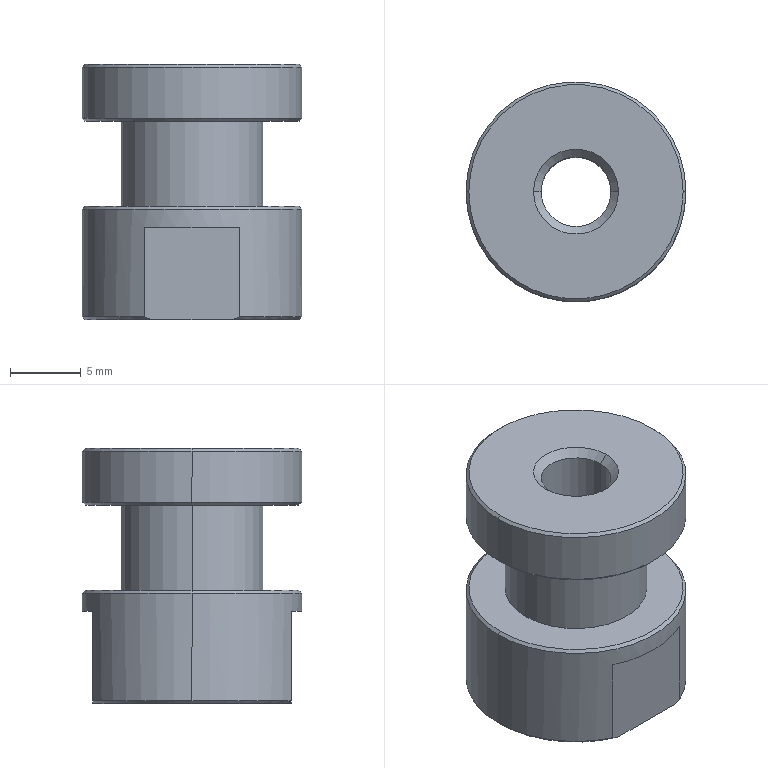Part | SolidWorks | features BaseBody 1 | 1 solid | 29 faces | box 15.5 x 15.5 x 18 mm | volume 2342 mm3 | cone 13 | cylinder 8 | plane 8 | commonest cylinder face diameters 15.5 x4 4.917 x2 10 x2
STEP:
#1=CARTESIAN_POINT('',(-2.458,0.,-17.459));
#2=VERTEX_POINT('',#1);
#3=CARTESIAN_POINT('',(2.458,0.,-17.459));
#4=VERTEX_POINT('',#3);
#5=CARTESIAN_POINT('',(0.,0.,-17.459));
#6=DIRECTION('',(0.,0.,1.));
#7=DIRECTION('',(1.,0.,0.));
#8=AXIS2_PLACEMENT_3D('',#5,#6,#7);
#9=CIRCLE('',#8,2.458);
#10=EDGE_CURVE('',#2,#4,#9,.T.);
#11=ORIENTED_EDGE('',*,*,#10,.T.);
#12=CARTESIAN_POINT('',(3.,0.,-18.));
#13=VERTEX_POINT('',#12);
#14=CARTESIAN_POINT('',(2.458,0.,-17.459));
#15=DIRECTION('',(0.7071,0.,-0.7071));
#16=VECTOR('',#15,1000.);
#17=LINE('',#14,#16);
#18=EDGE_CURVE('',#4,#13,#17,.T.);
#19=ORIENTED_EDGE('',*,*,#18,.T.);
#20=CARTESIAN_POINT('',(-3.,0.,-18.));
#21=VERTEX_POINT('',#20);
#22=CARTESIAN_POINT('',(0.,0.,-18.));
#23=DIRECTION('',(0.,0.,1.));
#24=DIRECTION('',(1.,0.,0.));
#25=AXIS2_PLACEMENT_3D('',#22,#23,#24);
#26=CIRCLE('',#25,3.);
#27=EDGE_CURVE('',#21,#13,#26,.T.);
#28=ORIENTED_EDGE('',*,*,#27,.F.);
#29=CARTESIAN_POINT('',(-2.458,0.,-17.459));
#30=DIRECTION('',(-0.7071,0.,-0.7071));
#31=VECTOR('',#30,1000.);
#32=LINE('',#29,#31);
#33=EDGE_CURVE('',#2,#21,#32,.T.);
#34=ORIENTED_EDGE('',*,*,#33,.F.);
#35=EDGE_LOOP('',(#11,#19,#28,#34));
#36=FACE_OUTER_BOUND('',#35,.T.);
#37=CARTESIAN_POINT('',(0.,0.,-17.459));
#38=DIRECTION('',(0.,0.,-1.));
#39=DIRECTION('',(-1.,0.,0.));
#40=AXIS2_PLACEMENT_3D('',#37,#38,#39);
#41=CONICAL_SURFACE('',#40,2.458,0.7854);
#42=ADVANCED_FACE('',(#36),#41,.F.);
#43=ORIENTED_EDGE('',*,*,#10,.F.);
#44=CARTESIAN_POINT('',(-2.458,0.,-0.5415));
#45=VERTEX_POINT('',#44);
#46=CARTESIAN_POINT('',(-2.458,0.,-50.));
#47=DIRECTION('',(0.,0.,1.));
#48=VECTOR('',#47,1000.);
#49=LINE('',#46,#48);
#50=EDGE_CURVE('',#2,#45,#49,.T.);
#51=ORIENTED_EDGE('',*,*,#50,.T.);
#52=CARTESIAN_POINT('',(2.458,0.,-0.5415));
#53=VERTEX_POINT('',#52);
#54=CARTESIAN_POINT('',(0.,0.,-0.5415));
#55=DIRECTION('',(0.,0.,1.));
#56=DIRECTION('',(1.,0.,0.));
#57=AXIS2_PLACEMENT_3D('',#54,#55,#56);
#58=CIRCLE('',#57,2.458);
#59=EDGE_CURVE('',#45,#53,#58,.T.);
#60=ORIENTED_EDGE('',*,*,#59,.T.);
#61=CARTESIAN_POINT('',(2.458,0.,-50.));
#62=DIRECTION('',(0.,0.,1.));
#63=VECTOR('',#62,1000.);
#64=LINE('',#61,#63);
#65=EDGE_CURVE('',#4,#53,#64,.T.);
#66=ORIENTED_EDGE('',*,*,#65,.F.);
#67=EDGE_LOOP('',(#43,#51,#60,#66));
#68=FACE_OUTER_BOUND('',#67,.T.);
#69=CARTESIAN_POINT('',(0.,0.,-50.));
#70=DIRECTION('',(0.,0.,1.));
#71=DIRECTION('',(1.,0.,0.));
#72=AXIS2_PLACEMENT_3D('',#69,#70,#71);
#73=CYLINDRICAL_SURFACE('',#72,2.458);
#74=ADVANCED_FACE('',(#68),#73,.F.);
#75=ORIENTED_EDGE('',*,*,#59,.F.);
#76=CARTESIAN_POINT('',(-3.,0.,0.));
#77=VERTEX_POINT('',#76);
#78=CARTESIAN_POINT('',(-3.,0.,0.));
#79=DIRECTION('',(-0.7071,0.,0.7071));
#80=VECTOR('',#79,1000.);
#81=LINE('',#78,#80);
#82=EDGE_CURVE('',#45,#77,#81,.T.);
#83=ORIENTED_EDGE('',*,*,#82,.T.);
#84=CARTESIAN_POINT('',(3.,0.,0.));
#85=VERTEX_POINT('',#84);
#86=CARTESIAN_POINT('',(0.,0.,0.));
#87=DIRECTION('',(0.,0.,1.));
#88=DIRECTION('',(1.,0.,0.));
#89=AXIS2_PLACEMENT_3D('',#86,#87,#88);
#90=CIRCLE('',#89,3.);
#91=EDGE_CURVE('',#77,#85,#90,.T.);
#92=ORIENTED_EDGE('',*,*,#91,.T.);
#93=CARTESIAN_POINT('',(3.,0.,0.));
#94=DIRECTION('',(0.7071,0.,0.7071));
#95=VECTOR('',#94,1000.);
#96=LINE('',#93,#95);
#97=EDGE_CURVE('',#53,#85,#96,.T.);
#98=ORIENTED_EDGE('',*,*,#97,.F.);
#99=EDGE_LOOP('',(#75,#83,#92,#98));
#100=FACE_OUTER_BOUND('',#99,.T.);
#101=CARTESIAN_POINT('',(0.,0.,0.));
#102=DIRECTION('',(0.,0.,1.));
#103=DIRECTION('',(1.,0.,0.));
#104=AXIS2_PLACEMENT_3D('',#101,#102,#103);
#105=CONICAL_SURFACE('',#104,3.,0.7854);
#106=ADVANCED_FACE('',(#100),#105,.F.);
#107=CARTESIAN_POINT('',(2.829,-7.,-18.));
#108=VERTEX_POINT('',#107);
#109=CARTESIAN_POINT('',(7.55,0.,-18.));
#110=VERTEX_POINT('',#109);
#111=CARTESIAN_POINT('',(0.,0.,-18.));
#112=DIRECTION('',(0.,0.,1.));
#113=DIRECTION('',(1.,0.,0.));
#114=AXIS2_PLACEMENT_3D('',#111,#112,#113);
#115=CIRCLE('',#114,7.55);
#116=EDGE_CURVE('',#108,#110,#115,.T.);
#117=ORIENTED_EDGE('',*,*,#116,.T.);
#118=CARTESIAN_POINT('',(7.75,0.,-17.8));
#119=VERTEX_POINT('',#118);
#120=CARTESIAN_POINT('',(7.75,0.,-17.8));
#121=DIRECTION('',(0.7071,0.,0.7071));
#122=VECTOR('',#121,1000.);
#123=LINE('',#120,#122);
#124=EDGE_CURVE('',#110,#119,#123,.T.);
#125=ORIENTED_EDGE('',*,*,#124,.T.);
#126=CARTESIAN_POINT('',(3.326,-7.,-17.8));
#127=VERTEX_POINT('',#126);
#128=CARTESIAN_POINT('',(0.,0.,-17.8));
#129=DIRECTION('',(0.,0.,1.));
#130=DIRECTION('',(1.,0.,0.));
#131=AXIS2_PLACEMENT_3D('',#128,#129,#130);
#132=CIRCLE('',#131,7.75);
#133=EDGE_CURVE('',#127,#119,#132,.T.);
#134=ORIENTED_EDGE('',*,*,#133,.F.);
#135=CARTESIAN_POINT('',(2.829,-7.,-18.));
#136=CARTESIAN_POINT('',(2.996,-7.,-17.937));
#137=CARTESIAN_POINT('',(3.161,-7.,-17.871));
#138=CARTESIAN_POINT('',(3.326,-7.,-17.8));
#139=B_SPLINE_CURVE_WITH_KNOTS('',3,(#135,#136,#137,#138),.UNSPECIFIED.,.F.,.F.,(4,4),(0.01089,0.01141),.UNSPECIFIED.);
#140=EDGE_CURVE('',#108,#127,#139,.T.);
#141=ORIENTED_EDGE('',*,*,#140,.F.);
#142=EDGE_LOOP('',(#117,#125,#134,#141));
#143=FACE_OUTER_BOUND('',#142,.T.);
#144=CARTESIAN_POINT('',(0.,0.,-17.8));
#145=DIRECTION('',(0.,0.,1.));
#146=DIRECTION('',(1.,0.,0.));
#147=AXIS2_PLACEMENT_3D('',#144,#145,#146);
#148=CONICAL_SURFACE('',#147,7.75,0.7854);
#149=ADVANCED_FACE('',(#143),#148,.T.);
#150=CARTESIAN_POINT('',(-3.326,7.,-17.8));
#151=VERTEX_POINT('',#150);
#152=CARTESIAN_POINT('',(-7.75,0.,-17.8));
#153=VERTEX_POINT('',#152);
#154=CARTESIAN_POINT('',(0.,0.,-17.8));
#155=DIRECTION('',(0.,0.,1.));
#156=DIRECTION('',(1.,0.,0.));
#157=AXIS2_PLACEMENT_3D('',#154,#155,#156);
#158=CIRCLE('',#157,7.75);
#159=EDGE_CURVE('',#151,#153,#158,.T.);
#160=ORIENTED_EDGE('',*,*,#159,.T.);
#161=CARTESIAN_POINT('',(-7.75,0.,-10.2));
#162=VERTEX_POINT('',#161);
#163=CARTESIAN_POINT('',(-7.75,0.,-50.));
#164=DIRECTION('',(0.,0.,1.));
#165=VECTOR('',#164,1000.);
#166=LINE('',#163,#165);
#167=EDGE_CURVE('',#153,#162,#166,.T.);
#168=ORIENTED_EDGE('',*,*,#167,.T.);
#169=CARTESIAN_POINT('',(7.75,0.,-10.2));
#170=VERTEX_POINT('',#169);
#171=CARTESIAN_POINT('',(0.,0.,-10.2));
#172=DIRECTION('',(0.,0.,1.));
#173=DIRECTION('',(1.,0.,0.));
#174=AXIS2_PLACEMENT_3D('',#171,#172,#173);
#175=CIRCLE('',#174,7.75);
#176=EDGE_CURVE('',#170,#162,#175,.T.);
#177=ORIENTED_EDGE('',*,*,#176,.F.);
#178=CARTESIAN_POINT('',(7.75,0.,-50.));
#179=DIRECTION('',(0.,0.,1.));
#180=VECTOR('',#179,1000.);
#181=LINE('',#178,#180);
#182=EDGE_CURVE('',#119,#170,#181,.T.);
#183=ORIENTED_EDGE('',*,*,#182,.F.);
#184=CARTESIAN_POINT('',(3.326,7.,-17.8));
#185=VERTEX_POINT('',#184);
#186=CARTESIAN_POINT('',(0.,0.,-17.8));
#187=DIRECTION('',(0.,0.,1.));
#188=DIRECTION('',(1.,0.,0.));
#189=AXIS2_PLACEMENT_3D('',#186,#187,#188);
#190=CIRCLE('',#189,7.75);
#191=EDGE_CURVE('',#119,#185,#190,.T.);
#192=ORIENTED_EDGE('',*,*,#191,.T.);
#193=CARTESIAN_POINT('',(3.326,7.,-11.5));
#194=VERTEX_POINT('',#193);
#195=CARTESIAN_POINT('',(3.326,7.,-11.5));
#196=DIRECTION('',(0.,0.,-1.));
#197=VECTOR('',#196,1000.);
#198=LINE('',#195,#197);
#199=EDGE_CURVE('',#194,#185,#198,.T.);
#200=ORIENTED_EDGE('',*,*,#199,.F.);
#201=CARTESIAN_POINT('',(-3.326,7.,-11.5));
#202=VERTEX_POINT('',#201);
#203=CARTESIAN_POINT('',(0.,0.,-11.5));
#204=DIRECTION('',(0.,0.,-1.));
#205=DIRECTION('',(1.,0.,0.));
#206=AXIS2_PLACEMENT_3D('',#203,#204,#205);
#207=CIRCLE('',#206,7.75);
#208=EDGE_CURVE('',#202,#194,#207,.T.);
#209=ORIENTED_EDGE('',*,*,#208,.F.);
#210=CARTESIAN_POINT('',(-3.326,7.,-11.5));
#211=DIRECTION('',(0.,0.,-1.));
#212=VECTOR('',#211,1000.);
#213=LINE('',#210,#212);
#214=EDGE_CURVE('',#202,#151,#213,.T.);
#215=ORIENTED_EDGE('',*,*,#214,.T.);
#216=EDGE_LOOP('',(#160,#168,#177,#183,#192,#200,#209,#215));
#217=FACE_OUTER_BOUND('',#216,.T.);
#218=CARTESIAN_POINT('',(0.,0.,-50.));
#219=DIRECTION('',(0.,0.,1.));
#220=DIRECTION('',(1.,0.,0.));
#221=AXIS2_PLACEMENT_3D('',#218,#219,#220);
#222=CYLINDRICAL_SURFACE('',#221,7.75);
#223=ADVANCED_FACE('',(#217),#222,.T.);
#224=CARTESIAN_POINT('',(7.55,0.,-10.));
#225=VERTEX_POINT('',#224);
#226=CARTESIAN_POINT('',(-7.55,0.,-10.));
#227=VERTEX_POINT('',#226);
#228=CARTESIAN_POINT('',(0.,0.,-10.));
#229=DIRECTION('',(0.,0.,1.));
#230=DIRECTION('',(1.,0.,0.));
#231=AXIS2_PLACEMENT_3D('',#228,#229,#230);
#232=CIRCLE('',#231,7.55);
#233=EDGE_CURVE('',#225,#227,#232,.T.);
#234=ORIENTED_EDGE('',*,*,#233,.F.);
#235=CARTESIAN_POINT('',(7.55,0.,-10.));
#236=DIRECTION('',(0.7071,0.,-0.7071));
#237=VECTOR('',#236,1000.);
#238=LINE('',#235,#237);
#239=EDGE_CURVE('',#225,#170,#238,.T.);
#240=ORIENTED_EDGE('',*,*,#239,.T.);
#241=ORIENTED_EDGE('',*,*,#176,.T.);
#242=CARTESIAN_POINT('',(-7.55,0.,-10.));
#243=DIRECTION('',(-0.7071,0.,-0.7071));
#244=VECTOR('',#243,1000.);
#245=LINE('',#242,#244);
#246=EDGE_CURVE('',#227,#162,#245,.T.);
#247=ORIENTED_EDGE('',*,*,#246,.F.);
#248=EDGE_LOOP('',(#234,#240,#241,#247));
#249=FACE_OUTER_BOUND('',#248,.T.);
#250=CARTESIAN_POINT('',(0.,0.,-10.));
#251=DIRECTION('',(0.,0.,-1.));
#252=DIRECTION('',(-1.,0.,0.));
#253=AXIS2_PLACEMENT_3D('',#250,#251,#252);
#254=CONICAL_SURFACE('',#253,7.55,0.7854);
#255=ADVANCED_FACE('',(#249),#254,.T.);
#256=CARTESIAN_POINT('',(5.,0.,-10.));
#257=VERTEX_POINT('',#256);
#258=CARTESIAN_POINT('',(-5.,0.,-10.));
#259=VERTEX_POINT('',#258);
#260=CARTESIAN_POINT('',(0.,0.,-10.));
#261=DIRECTION('',(0.,0.,1.));
#262=DIRECTION('',(1.,0.,0.));
#263=AXIS2_PLACEMENT_3D('',#260,#261,#262);
#264=CIRCLE('',#263,5.);
#265=EDGE_CURVE('',#257,#259,#264,.T.);
#266=ORIENTED_EDGE('',*,*,#265,.T.);
#267=CARTESIAN_POINT('',(-5.,0.,-4.));
#268=VERTEX_POINT('',#267);
#269=CARTESIAN_POINT('',(-5.,0.,-50.));
#270=DIRECTION('',(0.,0.,1.));
#271=VECTOR('',#270,1000.);
#272=LINE('',#269,#271);
#273=EDGE_CURVE('',#259,#268,#272,.T.);
#274=ORIENTED_EDGE('',*,*,#273,.T.);
#275=CARTESIAN_POINT('',(5.,0.,-4.));
#276=VERTEX_POINT('',#275);
#277=CARTESIAN_POINT('',(0.,0.,-4.));
#278=DIRECTION('',(0.,0.,1.));
#279=DIRECTION('',(1.,0.,0.));
#280=AXIS2_PLACEMENT_3D('',#277,#278,#279);
#281=CIRCLE('',#280,5.);
#282=EDGE_CURVE('',#276,#268,#281,.T.);
#283=ORIENTED_EDGE('',*,*,#282,.F.);
#284=CARTESIAN_POINT('',(5.,0.,-50.));
#285=DIRECTION('',(0.,0.,1.));
#286=VECTOR('',#285,1000.);
#287=LINE('',#284,#286);
#288=EDGE_CURVE('',#257,#276,#287,.T.);
#289=ORIENTED_EDGE('',*,*,#288,.F.);
#290=EDGE_LOOP('',(#266,#274,#283,#289));
#291=FACE_OUTER_BOUND('',#290,.T.);
#292=CARTESIAN_POINT('',(0.,0.,-50.));
#293=DIRECTION('',(0.,0.,1.));
#294=DIRECTION('',(1.,0.,0.));
#295=AXIS2_PLACEMENT_3D('',#292,#293,#294);
#296=CYLINDRICAL_SURFACE('',#295,5.);
#297=ADVANCED_FACE('',(#291),#296,.T.);
#298=CARTESIAN_POINT('',(7.55,0.,-4.));
#299=VERTEX_POINT('',#298);
#300=CARTESIAN_POINT('',(-7.55,0.,-4.));
#301=VERTEX_POINT('',#300);
#302=CARTESIAN_POINT('',(0.,0.,-4.));
#303=DIRECTION('',(0.,0.,1.));
#304=DIRECTION('',(1.,0.,0.));
#305=AXIS2_PLACEMENT_3D('',#302,#303,#304);
#306=CIRCLE('',#305,7.55);
#307=EDGE_CURVE('',#299,#301,#306,.T.);
#308=ORIENTED_EDGE('',*,*,#307,.T.);
#309=CARTESIAN_POINT('',(-7.75,0.,-3.8));
#310=VERTEX_POINT('',#309);
#311=CARTESIAN_POINT('',(-7.75,0.,-3.8));
#312=DIRECTION('',(-0.7071,0.,0.7071));
#313=VECTOR('',#312,1000.);
#314=LINE('',#311,#313);
#315=EDGE_CURVE('',#301,#310,#314,.T.);
#316=ORIENTED_EDGE('',*,*,#315,.T.);
#317=CARTESIAN_POINT('',(7.75,0.,-3.8));
#318=VERTEX_POINT('',#317);
#319=CARTESIAN_POINT('',(0.,0.,-3.8));
#320=DIRECTION('',(0.,0.,1.));
#321=DIRECTION('',(1.,0.,0.));
#322=AXIS2_PLACEMENT_3D('',#319,#320,#321);
#323=CIRCLE('',#322,7.75);
#324=EDGE_CURVE('',#318,#310,#323,.T.);
#325=ORIENTED_EDGE('',*,*,#324,.F.);
#326=CARTESIAN_POINT('',(7.75,0.,-3.8));
#327=DIRECTION('',(0.7071,0.,0.7071));
#328=VECTOR('',#327,1000.);
#329=LINE('',#326,#328);
#330=EDGE_CURVE('',#299,#318,#329,.T.);
#331=ORIENTED_EDGE('',*,*,#330,.F.);
#332=EDGE_LOOP('',(#308,#316,#325,#331));
#333=FACE_OUTER_BOUND('',#332,.T.);
#334=CARTESIAN_POINT('',(0.,0.,-3.8));
#335=DIRECTION('',(0.,0.,1.));
#336=DIRECTION('',(1.,0.,0.));
#337=AXIS2_PLACEMENT_3D('',#334,#335,#336);
#338=CONICAL_SURFACE('',#337,7.75,0.7854);
#339=ADVANCED_FACE('',(#333),#338,.T.);
#340=ORIENTED_EDGE('',*,*,#324,.T.);
#341=CARTESIAN_POINT('',(-7.75,0.,-0.2));
#342=VERTEX_POINT('',#341);
#343=CARTESIAN_POINT('',(-7.75,0.,-50.));
#344=DIRECTION('',(0.,0.,1.));
#345=VECTOR('',#344,1000.);
#346=LINE('',#343,#345);
#347=EDGE_CURVE('',#310,#342,#346,.T.);
#348=ORIENTED_EDGE('',*,*,#347,.T.);
#349=CARTESIAN_POINT('',(7.75,0.,-0.2));
#350=VERTEX_POINT('',#349);
#351=CARTESIAN_POINT('',(0.,0.,-0.2));
#352=DIRECTION('',(0.,0.,1.));
#353=DIRECTION('',(1.,0.,0.));
#354=AXIS2_PLACEMENT_3D('',#351,#352,#353);
#355=CIRCLE('',#354,7.75);
#356=EDGE_CURVE('',#350,#342,#355,.T.);
#357=ORIENTED_EDGE('',*,*,#356,.F.);
#358=CARTESIAN_POINT('',(7.75,0.,-50.));
#359=DIRECTION('',(0.,0.,1.));
#360=VECTOR('',#359,1000.);
#361=LINE('',#358,#360);
#362=EDGE_CURVE('',#318,#350,#361,.T.);
#363=ORIENTED_EDGE('',*,*,#362,.F.);
#364=EDGE_LOOP('',(#340,#348,#357,#363));
#365=FACE_OUTER_BOUND('',#364,.T.);
#366=CARTESIAN_POINT('',(0.,0.,-50.));
#367=DIRECTION('',(0.,0.,1.));
#368=DIRECTION('',(1.,0.,0.));
#369=AXIS2_PLACEMENT_3D('',#366,#367,#368);
#370=CYLINDRICAL_SURFACE('',#369,7.75);
#371=ADVANCED_FACE('',(#365),#370,.T.);
#372=CARTESIAN_POINT('',(7.55,0.,0.));
#373=VERTEX_POINT('',#372);
#374=CARTESIAN_POINT('',(-7.55,0.,0.));
#375=VERTEX_POINT('',#374);
#376=CARTESIAN_POINT('',(0.,0.,0.));
#377=DIRECTION('',(0.,0.,1.));
#378=DIRECTION('',(1.,0.,0.));
#379=AXIS2_PLACEMENT_3D('',#376,#377,#378);
#380=CIRCLE('',#379,7.55);
#381=EDGE_CURVE('',#373,#375,#380,.T.);
#382=ORIENTED_EDGE('',*,*,#381,.F.);
#383=CARTESIAN_POINT('',(7.55,0.,0.));
#384=DIRECTION('',(0.7071,0.,-0.7071));
#385=VECTOR('',#384,1000.);
#386=LINE('',#383,#385);
#387=EDGE_CURVE('',#373,#350,#386,.T.);
#388=ORIENTED_EDGE('',*,*,#387,.T.);
#389=ORIENTED_EDGE('',*,*,#356,.T.);
#390=CARTESIAN_POINT('',(-7.55,0.,0.));
#391=DIRECTION('',(-0.7071,0.,-0.7071));
#392=VECTOR('',#391,1000.);
#393=LINE('',#390,#392);
#394=EDGE_CURVE('',#375,#342,#393,.T.);
#395=ORIENTED_EDGE('',*,*,#394,.F.);
#396=EDGE_LOOP('',(#382,#388,#389,#395));
#397=FACE_OUTER_BOUND('',#396,.T.);
#398=CARTESIAN_POINT('',(0.,0.,0.));
#399=DIRECTION('',(0.,0.,-1.));
#400=DIRECTION('',(-1.,0.,0.));
#401=AXIS2_PLACEMENT_3D('',#398,#399,#400);
#402=CONICAL_SURFACE('',#401,7.55,0.7854);
#403=ADVANCED_FACE('',(#397),#402,.T.);
#404=CARTESIAN_POINT('',(-3.326,-7.,-17.8));
#405=VERTEX_POINT('',#404);
#406=CARTESIAN_POINT('',(-2.829,-7.,-18.));
#407=VERTEX_POINT('',#406);
#408=CARTESIAN_POINT('',(-3.326,-7.,-17.8));
#409=CARTESIAN_POINT('',(-3.162,-7.,-17.87));
#410=CARTESIAN_POINT('',(-2.997,-7.,-17.937));
#411=CARTESIAN_POINT('',(-2.829,-7.,-18.));
#412=B_SPLINE_CURVE_WITH_KNOTS('',3,(#408,#409,#410,#411),.UNSPECIFIED.,.F.,.F.,(4,4),(0.004643,0.005176),.UNSPECIFIED.);
#413=EDGE_CURVE('',#405,#407,#412,.T.);
#414=ORIENTED_EDGE('',*,*,#413,.F.);
#415=CARTESIAN_POINT('',(0.,0.,-17.8));
#416=DIRECTION('',(0.,0.,1.));
#417=DIRECTION('',(1.,0.,0.));
#418=AXIS2_PLACEMENT_3D('',#415,#416,#417);
#419=CIRCLE('',#418,7.75);
#420=EDGE_CURVE('',#153,#405,#419,.T.);
#421=ORIENTED_EDGE('',*,*,#420,.F.);
#422=ORIENTED_EDGE('',*,*,#159,.F.);
#423=CARTESIAN_POINT('',(-2.829,7.,-18.));
#424=VERTEX_POINT('',#423);
#425=CARTESIAN_POINT('',(-2.829,7.,-18.));
#426=CARTESIAN_POINT('',(-2.996,7.,-17.937));
#427=CARTESIAN_POINT('',(-3.161,7.,-17.871));
#428=CARTESIAN_POINT('',(-3.326,7.,-17.8));
#429=B_SPLINE_CURVE_WITH_KNOTS('',3,(#425,#426,#427,#428),.UNSPECIFIED.,.F.,.F.,(4,4),(0.01089,0.01141),.UNSPECIFIED.);
#430=EDGE_CURVE('',#424,#151,#429,.T.);
#431=ORIENTED_EDGE('',*,*,#430,.F.);
#432=CARTESIAN_POINT('',(0.,0.,-18.));
#433=DIRECTION('',(0.,0.,1.));
#434=DIRECTION('',(1.,0.,0.));
#435=AXIS2_PLACEMENT_3D('',#432,#433,#434);
#436=CIRCLE('',#435,7.55);
#437=EDGE_CURVE('',#424,#407,#436,.T.);
#438=ORIENTED_EDGE('',*,*,#437,.T.);
#439=EDGE_LOOP('',(#414,#421,#422,#431,#438));
#440=FACE_OUTER_BOUND('',#439,.T.);
#441=CARTESIAN_POINT('',(0.,0.,-17.8));
#442=DIRECTION('',(0.,0.,1.));
#443=DIRECTION('',(1.,0.,0.));
#444=AXIS2_PLACEMENT_3D('',#441,#442,#443);
#445=CONICAL_SURFACE('',#444,7.75,0.7854);
#446=ADVANCED_FACE('',(#440),#445,.T.);
#447=CARTESIAN_POINT('',(0.,0.,0.));
#448=DIRECTION('',(0.,0.,1.));
#449=DIRECTION('',(1.,0.,0.));
#450=AXIS2_PLACEMENT_3D('',#447,#448,#449);
#451=CIRCLE('',#450,3.);
#452=EDGE_CURVE('',#85,#77,#451,.T.);
#453=ORIENTED_EDGE('',*,*,#452,.F.);
#454=ORIENTED_EDGE('',*,*,#91,.F.);
#455=EDGE_LOOP('',(#453,#454));
#456=FACE_BOUND('',#455,.T.);
#457=CARTESIAN_POINT('',(0.,0.,0.));
#458=DIRECTION('',(0.,0.,1.));
#459=DIRECTION('',(1.,0.,0.));
#460=AXIS2_PLACEMENT_3D('',#457,#458,#459);
#461=CIRCLE('',#460,7.55);
#462=EDGE_CURVE('',#375,#373,#461,.T.);
#463=ORIENTED_EDGE('',*,*,#462,.T.);
#464=ORIENTED_EDGE('',*,*,#381,.T.);
#465=EDGE_LOOP('',(#463,#464));
#466=FACE_OUTER_BOUND('',#465,.T.);
#467=CARTESIAN_POINT('',(0.,0.,0.));
#468=DIRECTION('',(0.,0.,1.));
#469=DIRECTION('',(1.,0.,0.));
#470=AXIS2_PLACEMENT_3D('',#467,#468,#469);
#471=PLANE('',#470);
#472=ADVANCED_FACE('',(#456,#466),#471,.T.);
#473=ORIENTED_EDGE('',*,*,#387,.F.);
#474=ORIENTED_EDGE('',*,*,#462,.F.);
#475=ORIENTED_EDGE('',*,*,#394,.T.);
#476=CARTESIAN_POINT('',(0.,0.,-0.2));
#477=DIRECTION('',(0.,0.,1.));
#478=DIRECTION('',(1.,0.,0.));
#479=AXIS2_PLACEMENT_3D('',#476,#477,#478);
#480=CIRCLE('',#479,7.75);
#481=EDGE_CURVE('',#342,#350,#480,.T.);
#482=ORIENTED_EDGE('',*,*,#481,.T.);
#483=EDGE_LOOP('',(#473,#474,#475,#482));
#484=FACE_OUTER_BOUND('',#483,.T.);
#485=CARTESIAN_POINT('',(0.,0.,0.));
#486=DIRECTION('',(0.,0.,-1.));
#487=DIRECTION('',(-1.,0.,0.));
#488=AXIS2_PLACEMENT_3D('',#485,#486,#487);
#489=CONICAL_SURFACE('',#488,7.55,0.7854);
#490=ADVANCED_FACE('',(#484),#489,.T.);
#491=ORIENTED_EDGE('',*,*,#347,.F.);
#492=CARTESIAN_POINT('',(0.,0.,-3.8));
#493=DIRECTION('',(0.,0.,1.));
#494=DIRECTION('',(1.,0.,0.));
#495=AXIS2_PLACEMENT_3D('',#492,#493,#494);
#496=CIRCLE('',#495,7.75);
#497=EDGE_CURVE('',#310,#318,#496,.T.);
#498=ORIENTED_EDGE('',*,*,#497,.T.);
#499=ORIENTED_EDGE('',*,*,#362,.T.);
#500=ORIENTED_EDGE('',*,*,#481,.F.);
#501=EDGE_LOOP('',(#491,#498,#499,#500));
#502=FACE_OUTER_BOUND('',#501,.T.);
#503=CARTESIAN_POINT('',(0.,0.,-50.));
#504=DIRECTION('',(0.,0.,1.));
#505=DIRECTION('',(1.,0.,0.));
#506=AXIS2_PLACEMENT_3D('',#503,#504,#505);
#507=CYLINDRICAL_SURFACE('',#506,7.75);
#508=ADVANCED_FACE('',(#502),#507,.T.);
#509=ORIENTED_EDGE('',*,*,#315,.F.);
#510=CARTESIAN_POINT('',(0.,0.,-4.));
#511=DIRECTION('',(0.,0.,1.));
#512=DIRECTION('',(1.,0.,0.));
#513=AXIS2_PLACEMENT_3D('',#510,#511,#512);
#514=CIRCLE('',#513,7.55);
#515=EDGE_CURVE('',#301,#299,#514,.T.);
#516=ORIENTED_EDGE('',*,*,#515,.T.);
#517=ORIENTED_EDGE('',*,*,#330,.T.);
#518=ORIENTED_EDGE('',*,*,#497,.F.);
#519=EDGE_LOOP('',(#509,#516,#517,#518));
#520=FACE_OUTER_BOUND('',#519,.T.);
#521=CARTESIAN_POINT('',(0.,0.,-3.8));
#522=DIRECTION('',(0.,0.,1.));
#523=DIRECTION('',(1.,0.,0.));
#524=AXIS2_PLACEMENT_3D('',#521,#522,#523);
#525=CONICAL_SURFACE('',#524,7.75,0.7854);
#526=ADVANCED_FACE('',(#520),#525,.T.);
#527=ORIENTED_EDGE('',*,*,#282,.T.);
#528=CARTESIAN_POINT('',(0.,0.,-4.));
#529=DIRECTION('',(0.,0.,1.));
#530=DIRECTION('',(1.,0.,0.));
#531=AXIS2_PLACEMENT_3D('',#528,#529,#530);
#532=CIRCLE('',#531,5.);
#533=EDGE_CURVE('',#268,#276,#532,.T.);
#534=ORIENTED_EDGE('',*,*,#533,.T.);
#535=EDGE_LOOP('',(#527,#534));
#536=FACE_BOUND('',#535,.T.);
#537=ORIENTED_EDGE('',*,*,#307,.F.);
#538=ORIENTED_EDGE('',*,*,#515,.F.);
#539=EDGE_LOOP('',(#537,#538));
#540=FACE_OUTER_BOUND('',#539,.T.);
#541=CARTESIAN_POINT('',(0.,7.55,-4.));
#542=DIRECTION('',(0.,0.,-1.));
#543=DIRECTION('',(-1.,0.,0.));
#544=AXIS2_PLACEMENT_3D('',#541,#542,#543);
#545=PLANE('',#544);
#546=ADVANCED_FACE('',(#536,#540),#545,.T.);
#547=ORIENTED_EDGE('',*,*,#273,.F.);
#548=CARTESIAN_POINT('',(0.,0.,-10.));
#549=DIRECTION('',(0.,0.,1.));
#550=DIRECTION('',(1.,0.,0.));
#551=AXIS2_PLACEMENT_3D('',#548,#549,#550);
#552=CIRCLE('',#551,5.);
#553=EDGE_CURVE('',#259,#257,#552,.T.);
#554=ORIENTED_EDGE('',*,*,#553,.T.);
#555=ORIENTED_EDGE('',*,*,#288,.T.);
#556=ORIENTED_EDGE('',*,*,#533,.F.);
#557=EDGE_LOOP('',(#547,#554,#555,#556));
#558=FACE_OUTER_BOUND('',#557,.T.);
#559=CARTESIAN_POINT('',(0.,0.,-50.));
#560=DIRECTION('',(0.,0.,1.));
#561=DIRECTION('',(1.,0.,0.));
#562=AXIS2_PLACEMENT_3D('',#559,#560,#561);
#563=CYLINDRICAL_SURFACE('',#562,5.);
#564=ADVANCED_FACE('',(#558),#563,.T.);
#565=CARTESIAN_POINT('',(0.,0.,-10.));
#566=DIRECTION('',(0.,0.,1.));
#567=DIRECTION('',(1.,0.,0.));
#568=AXIS2_PLACEMENT_3D('',#565,#566,#567);
#569=CIRCLE('',#568,7.55);
#570=EDGE_CURVE('',#227,#225,#569,.T.);
#571=ORIENTED_EDGE('',*,*,#570,.T.);
#572=ORIENTED_EDGE('',*,*,#233,.T.);
#573=EDGE_LOOP('',(#571,#572));
#574=FACE_OUTER_BOUND('',#573,.T.);
#575=ORIENTED_EDGE('',*,*,#265,.F.);
#576=ORIENTED_EDGE('',*,*,#553,.F.);
#577=EDGE_LOOP('',(#575,#576));
#578=FACE_BOUND('',#577,.T.);
#579=CARTESIAN_POINT('',(0.,5.,-10.));
#580=DIRECTION('',(0.,0.,1.));
#581=DIRECTION('',(1.,0.,0.));
#582=AXIS2_PLACEMENT_3D('',#579,#580,#581);
#583=PLANE('',#582);
#584=ADVANCED_FACE('',(#574,#578),#583,.T.);
#585=ORIENTED_EDGE('',*,*,#239,.F.);
#586=ORIENTED_EDGE('',*,*,#570,.F.);
#587=ORIENTED_EDGE('',*,*,#246,.T.);
#588=CARTESIAN_POINT('',(0.,0.,-10.2));
#589=DIRECTION('',(0.,0.,1.));
#590=DIRECTION('',(1.,0.,0.));
#591=AXIS2_PLACEMENT_3D('',#588,#589,#590);
#592=CIRCLE('',#591,7.75);
#593=EDGE_CURVE('',#162,#170,#592,.T.);
#594=ORIENTED_EDGE('',*,*,#593,.T.);
#595=EDGE_LOOP('',(#585,#586,#587,#594));
#596=FACE_OUTER_BOUND('',#595,.T.);
#597=CARTESIAN_POINT('',(0.,0.,-10.));
#598=DIRECTION('',(0.,0.,-1.));
#599=DIRECTION('',(-1.,0.,0.));
#600=AXIS2_PLACEMENT_3D('',#597,#598,#599);
#601=CONICAL_SURFACE('',#600,7.55,0.7854);
#602=ADVANCED_FACE('',(#596),#601,.T.);
#603=ORIENTED_EDGE('',*,*,#167,.F.);
#604=ORIENTED_EDGE('',*,*,#420,.T.);
#605=CARTESIAN_POINT('',(-3.326,-7.,-11.5));
#606=VERTEX_POINT('',#605);
#607=CARTESIAN_POINT('',(-3.326,-7.,-11.5));
#608=DIRECTION('',(0.,0.,-1.));
#609=VECTOR('',#608,1000.);
#610=LINE('',#607,#609);
#611=EDGE_CURVE('',#606,#405,#610,.T.);
#612=ORIENTED_EDGE('',*,*,#611,.F.);
#613=CARTESIAN_POINT('',(3.326,-7.,-11.5));
#614=VERTEX_POINT('',#613);
#615=CARTESIAN_POINT('',(0.,0.,-11.5));
#616=DIRECTION('',(0.,0.,-1.));
#617=DIRECTION('',(1.,0.,0.));
#618=AXIS2_PLACEMENT_3D('',#615,#616,#617);
#619=CIRCLE('',#618,7.75);
#620=EDGE_CURVE('',#614,#606,#619,.T.);
#621=ORIENTED_EDGE('',*,*,#620,.F.);
#622=CARTESIAN_POINT('',(3.326,-7.,-11.5));
#623=DIRECTION('',(0.,0.,-1.));
#624=VECTOR('',#623,1000.);
#625=LINE('',#622,#624);
#626=EDGE_CURVE('',#614,#127,#625,.T.);
#627=ORIENTED_EDGE('',*,*,#626,.T.);
#628=ORIENTED_EDGE('',*,*,#133,.T.);
#629=ORIENTED_EDGE('',*,*,#182,.T.);
#630=ORIENTED_EDGE('',*,*,#593,.F.);
#631=EDGE_LOOP('',(#603,#604,#612,#621,#627,#628,#629,#630));
#632=FACE_OUTER_BOUND('',#631,.T.);
#633=CARTESIAN_POINT('',(0.,0.,-50.));
#634=DIRECTION('',(0.,0.,1.));
#635=DIRECTION('',(1.,0.,0.));
#636=AXIS2_PLACEMENT_3D('',#633,#634,#635);
#637=CYLINDRICAL_SURFACE('',#636,7.75);
#638=ADVANCED_FACE('',(#632),#637,.T.);
#639=ORIENTED_EDGE('',*,*,#124,.F.);
#640=CARTESIAN_POINT('',(2.829,7.,-18.));
#641=VERTEX_POINT('',#640);
#642=CARTESIAN_POINT('',(0.,0.,-18.));
#643=DIRECTION('',(0.,0.,1.));
#644=DIRECTION('',(1.,0.,0.));
#645=AXIS2_PLACEMENT_3D('',#642,#643,#644);
#646=CIRCLE('',#645,7.55);
#647=EDGE_CURVE('',#110,#641,#646,.T.);
#648=ORIENTED_EDGE('',*,*,#647,.T.);
#649=CARTESIAN_POINT('',(3.326,7.,-17.8));
#650=CARTESIAN_POINT('',(3.162,7.,-17.87));
#651=CARTESIAN_POINT('',(2.997,7.,-17.937));
#652=CARTESIAN_POINT('',(2.829,7.,-18.));
#653=B_SPLINE_CURVE_WITH_KNOTS('',3,(#649,#650,#651,#652),.UNSPECIFIED.,.F.,.F.,(4,4),(0.004643,0.005176),.UNSPECIFIED.);
#654=EDGE_CURVE('',#185,#641,#653,.T.);
#655=ORIENTED_EDGE('',*,*,#654,.F.);
#656=ORIENTED_EDGE('',*,*,#191,.F.);
#657=EDGE_LOOP('',(#639,#648,#655,#656));
#658=FACE_OUTER_BOUND('',#657,.T.);
#659=CARTESIAN_POINT('',(0.,0.,-17.8));
#660=DIRECTION('',(0.,0.,1.));
#661=DIRECTION('',(1.,0.,0.));
#662=AXIS2_PLACEMENT_3D('',#659,#660,#661);
#663=CONICAL_SURFACE('',#662,7.75,0.7854);
#664=ADVANCED_FACE('',(#658),#663,.T.);
#665=ORIENTED_EDGE('',*,*,#27,.T.);
#666=CARTESIAN_POINT('',(0.,0.,-18.));
#667=DIRECTION('',(0.,0.,1.));
#668=DIRECTION('',(1.,0.,0.));
#669=AXIS2_PLACEMENT_3D('',#666,#667,#668);
#670=CIRCLE('',#669,3.);
#671=EDGE_CURVE('',#13,#21,#670,.T.);
#672=ORIENTED_EDGE('',*,*,#671,.T.);
#673=EDGE_LOOP('',(#665,#672));
#674=FACE_BOUND('',#673,.T.);
#675=CARTESIAN_POINT('',(-3.326,-7.,-18.));
#676=DIRECTION('',(1.,0.,0.));
#677=VECTOR('',#676,1000.);
#678=LINE('',#675,#677);
#679=EDGE_CURVE('',#407,#108,#678,.T.);
#680=ORIENTED_EDGE('',*,*,#679,.F.);
#681=ORIENTED_EDGE('',*,*,#437,.F.);
#682=CARTESIAN_POINT('',(3.326,7.,-18.));
#683=DIRECTION('',(-1.,0.,0.));
#684=VECTOR('',#683,1000.);
#685=LINE('',#682,#684);
#686=EDGE_CURVE('',#641,#424,#685,.T.);
#687=ORIENTED_EDGE('',*,*,#686,.F.);
#688=ORIENTED_EDGE('',*,*,#647,.F.);
#689=ORIENTED_EDGE('',*,*,#116,.F.);
#690=EDGE_LOOP('',(#680,#681,#687,#688,#689));
#691=FACE_OUTER_BOUND('',#690,.T.);
#692=CARTESIAN_POINT('',(0.,7.55,-18.));
#693=DIRECTION('',(0.,0.,-1.));
#694=DIRECTION('',(-1.,0.,0.));
#695=AXIS2_PLACEMENT_3D('',#692,#693,#694);
#696=PLANE('',#695);
#697=ADVANCED_FACE('',(#674,#691),#696,.T.);
#698=ORIENTED_EDGE('',*,*,#654,.T.);
#699=ORIENTED_EDGE('',*,*,#686,.T.);
#700=ORIENTED_EDGE('',*,*,#430,.T.);
#701=ORIENTED_EDGE('',*,*,#214,.F.);
#702=CARTESIAN_POINT('',(3.326,7.,-11.5));
#703=DIRECTION('',(-1.,0.,0.));
#704=VECTOR('',#703,1000.);
#705=LINE('',#702,#704);
#706=EDGE_CURVE('',#194,#202,#705,.T.);
#707=ORIENTED_EDGE('',*,*,#706,.F.);
#708=ORIENTED_EDGE('',*,*,#199,.T.);
#709=EDGE_LOOP('',(#698,#699,#700,#701,#707,#708));
#710=FACE_OUTER_BOUND('',#709,.T.);
#711=CARTESIAN_POINT('',(3.326,7.,-11.5));
#712=DIRECTION('',(0.,-1.,0.));
#713=DIRECTION('',(0.,0.,-1.));
#714=AXIS2_PLACEMENT_3D('',#711,#712,#713);
#715=PLANE('',#714);
#716=ADVANCED_FACE('',(#710),#715,.F.);
#717=ORIENTED_EDGE('',*,*,#208,.T.);
#718=ORIENTED_EDGE('',*,*,#706,.T.);
#719=EDGE_LOOP('',(#717,#718));
#720=FACE_OUTER_BOUND('',#719,.T.);
#721=CARTESIAN_POINT('',(0.,0.,-11.5));
#722=DIRECTION('',(0.,0.,-1.));
#723=DIRECTION('',(-1.,0.,0.));
#724=AXIS2_PLACEMENT_3D('',#721,#722,#723);
#725=PLANE('',#724);
#726=ADVANCED_FACE('',(#720),#725,.T.);
#727=ORIENTED_EDGE('',*,*,#413,.T.);
#728=ORIENTED_EDGE('',*,*,#679,.T.);
#729=ORIENTED_EDGE('',*,*,#140,.T.);
#730=ORIENTED_EDGE('',*,*,#626,.F.);
#731=CARTESIAN_POINT('',(-3.326,-7.,-11.5));
#732=DIRECTION('',(1.,0.,0.));
#733=VECTOR('',#732,1000.);
#734=LINE('',#731,#733);
#735=EDGE_CURVE('',#606,#614,#734,.T.);
#736=ORIENTED_EDGE('',*,*,#735,.F.);
#737=ORIENTED_EDGE('',*,*,#611,.T.);
#738=EDGE_LOOP('',(#727,#728,#729,#730,#736,#737));
#739=FACE_OUTER_BOUND('',#738,.T.);
#740=CARTESIAN_POINT('',(-3.326,-7.,-11.5));
#741=DIRECTION('',(0.,1.,0.));
#742=DIRECTION('',(0.,0.,1.));
#743=AXIS2_PLACEMENT_3D('',#740,#741,#742);
#744=PLANE('',#743);
#745=ADVANCED_FACE('',(#739),#744,.F.);
#746=ORIENTED_EDGE('',*,*,#735,.T.);
#747=ORIENTED_EDGE('',*,*,#620,.T.);
#748=EDGE_LOOP('',(#746,#747));
#749=FACE_OUTER_BOUND('',#748,.T.);
#750=CARTESIAN_POINT('',(0.,0.,-11.5));
#751=DIRECTION('',(0.,0.,-1.));
#752=DIRECTION('',(-1.,0.,0.));
#753=AXIS2_PLACEMENT_3D('',#750,#751,#752);
#754=PLANE('',#753);
#755=ADVANCED_FACE('',(#749),#754,.T.);
#756=ORIENTED_EDGE('',*,*,#82,.F.);
#757=CARTESIAN_POINT('',(0.,0.,-0.5415));
#758=DIRECTION('',(0.,0.,1.));
#759=DIRECTION('',(1.,0.,0.));
#760=AXIS2_PLACEMENT_3D('',#757,#758,#759);
#761=CIRCLE('',#760,2.458);
#762=EDGE_CURVE('',#53,#45,#761,.T.);
#763=ORIENTED_EDGE('',*,*,#762,.F.);
#764=ORIENTED_EDGE('',*,*,#97,.T.);
#765=ORIENTED_EDGE('',*,*,#452,.T.);
#766=EDGE_LOOP('',(#756,#763,#764,#765));
#767=FACE_OUTER_BOUND('',#766,.T.);
#768=CARTESIAN_POINT('',(0.,0.,0.));
#769=DIRECTION('',(0.,0.,1.));
#770=DIRECTION('',(1.,0.,0.));
#771=AXIS2_PLACEMENT_3D('',#768,#769,#770);
#772=CONICAL_SURFACE('',#771,3.,0.7854);
#773=ADVANCED_FACE('',(#767),#772,.F.);
#774=ORIENTED_EDGE('',*,*,#50,.F.);
#775=CARTESIAN_POINT('',(0.,0.,-17.459));
#776=DIRECTION('',(0.,0.,1.));
#777=DIRECTION('',(1.,0.,0.));
#778=AXIS2_PLACEMENT_3D('',#775,#776,#777);
#779=CIRCLE('',#778,2.458);
#780=EDGE_CURVE('',#4,#2,#779,.T.);
#781=ORIENTED_EDGE('',*,*,#780,.F.);
#782=ORIENTED_EDGE('',*,*,#65,.T.);
#783=ORIENTED_EDGE('',*,*,#762,.T.);
#784=EDGE_LOOP('',(#774,#781,#782,#783));
#785=FACE_OUTER_BOUND('',#784,.T.);
#786=CARTESIAN_POINT('',(0.,0.,-50.));
#787=DIRECTION('',(0.,0.,1.));
#788=DIRECTION('',(1.,0.,0.));
#789=AXIS2_PLACEMENT_3D('',#786,#787,#788);
#790=CYLINDRICAL_SURFACE('',#789,2.458);
#791=ADVANCED_FACE('',(#785),#790,.F.);
#792=ORIENTED_EDGE('',*,*,#18,.F.);
#793=ORIENTED_EDGE('',*,*,#780,.T.);
#794=ORIENTED_EDGE('',*,*,#33,.T.);
#795=ORIENTED_EDGE('',*,*,#671,.F.);
#796=EDGE_LOOP('',(#792,#793,#794,#795));
#797=FACE_OUTER_BOUND('',#796,.T.);
#798=CARTESIAN_POINT('',(0.,0.,-17.459));
#799=DIRECTION('',(0.,0.,-1.));
#800=DIRECTION('',(-1.,0.,0.));
#801=AXIS2_PLACEMENT_3D('',#798,#799,#800);
#802=CONICAL_SURFACE('',#801,2.458,0.7854);
#803=ADVANCED_FACE('',(#797),#802,.F.);
#804=CLOSED_SHELL('',(#42,#74,#106,#149,#223,#255,#297,#339,#371,#403,#446,#472,#490,#508,#526,#546,#564,#584,#602,#638,#664,#697,#716,#726,#745,#755,#773,#791,#803));
#805=MANIFOLD_SOLID_BREP('',#804);
#806=CARTESIAN_POINT('',(0.,0.,0.));
#807=DIRECTION('',(0.,0.,1.));
#808=DIRECTION('',(1.,0.,0.));
#809=AXIS2_PLACEMENT_3D('',#806,#807,#808);
#810=(LENGTH_UNIT()NAMED_UNIT(*)SI_UNIT(.MILLI.,.METRE.));
#811=UNCERTAINTY_MEASURE_WITH_UNIT(LENGTH_MEASURE(0.00001),#810,'','');
#812=(NAMED_UNIT(*)PLANE_ANGLE_UNIT()SI_UNIT($,.RADIAN.));
#813=(NAMED_UNIT(*)SI_UNIT($,.STERADIAN.)SOLID_ANGLE_UNIT());
#814=(GEOMETRIC_REPRESENTATION_CONTEXT(3)GLOBAL_UNCERTAINTY_ASSIGNED_CONTEXT((#811))GLOBAL_UNIT_ASSIGNED_CONTEXT((#810,#812,#813))REPRESENTATION_CONTEXT('',''));
#815=ADVANCED_BREP_SHAPE_REPRESENTATION('',(#805,#809),#814);